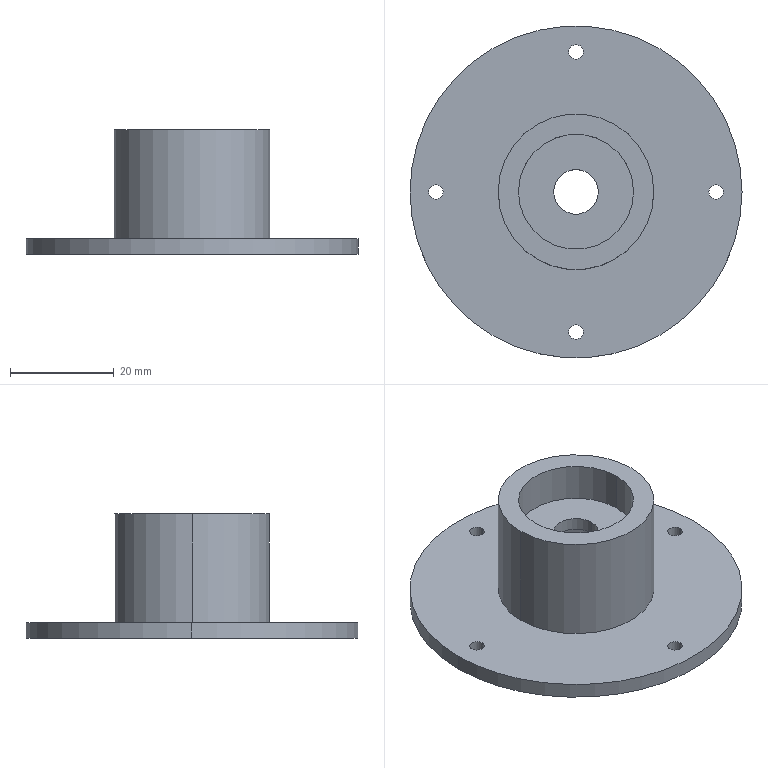Part | SolidWorks | features Fillet 1, HoleWzd 1, ICE 1, RevCut 1, Revolution 1 | 1 solid | 23 faces | box 64 x 64 x 24 mm | volume 13940 mm3 | cylinder 18 | plane 5 | commonest cylinder face diameters 2.8 x8 8.6 x2 22.2 x2 26 x2 30 x2 64 x2
STEP:
#1=CARTESIAN_POINT('',(-1.4,27.,0.));
#2=VERTEX_POINT('',#1);
#3=CARTESIAN_POINT('',(1.4,27.,0.));
#4=VERTEX_POINT('',#3);
#5=CARTESIAN_POINT('',(0.,27.,0.));
#6=DIRECTION('',(0.,0.,1.));
#7=DIRECTION('',(1.,0.,0.));
#8=AXIS2_PLACEMENT_3D('',#5,#6,#7);
#9=CIRCLE('',#8,1.4);
#10=EDGE_CURVE('',#2,#4,#9,.T.);
#11=ORIENTED_EDGE('',*,*,#10,.F.);
#12=CARTESIAN_POINT('',(-1.4,27.,3.));
#13=VERTEX_POINT('',#12);
#14=CARTESIAN_POINT('',(-1.4,27.,3.));
#15=DIRECTION('',(0.,0.,1.));
#16=VECTOR('',#15,1000.);
#17=LINE('',#14,#16);
#18=EDGE_CURVE('',#2,#13,#17,.T.);
#19=ORIENTED_EDGE('',*,*,#18,.T.);
#20=CARTESIAN_POINT('',(1.4,27.,3.));
#21=VERTEX_POINT('',#20);
#22=CARTESIAN_POINT('',(0.,27.,3.));
#23=DIRECTION('',(0.,0.,1.));
#24=DIRECTION('',(1.,0.,0.));
#25=AXIS2_PLACEMENT_3D('',#22,#23,#24);
#26=CIRCLE('',#25,1.4);
#27=EDGE_CURVE('',#13,#21,#26,.T.);
#28=ORIENTED_EDGE('',*,*,#27,.T.);
#29=CARTESIAN_POINT('',(1.4,27.,3.));
#30=DIRECTION('',(0.,0.,1.));
#31=VECTOR('',#30,1000.);
#32=LINE('',#29,#31);
#33=EDGE_CURVE('',#4,#21,#32,.T.);
#34=ORIENTED_EDGE('',*,*,#33,.F.);
#35=EDGE_LOOP('',(#11,#19,#28,#34));
#36=FACE_OUTER_BOUND('',#35,.T.);
#37=CARTESIAN_POINT('',(0.,27.,3.));
#38=DIRECTION('',(0.,0.,1.));
#39=DIRECTION('',(1.,0.,0.));
#40=AXIS2_PLACEMENT_3D('',#37,#38,#39);
#41=CYLINDRICAL_SURFACE('',#40,1.4);
#42=ADVANCED_FACE('',(#36),#41,.F.);
#43=CARTESIAN_POINT('',(-1.4,-27.,0.));
#44=VERTEX_POINT('',#43);
#45=CARTESIAN_POINT('',(1.4,-27.,0.));
#46=VERTEX_POINT('',#45);
#47=CARTESIAN_POINT('',(0.,-27.,0.));
#48=DIRECTION('',(0.,0.,1.));
#49=DIRECTION('',(1.,0.,0.));
#50=AXIS2_PLACEMENT_3D('',#47,#48,#49);
#51=CIRCLE('',#50,1.4);
#52=EDGE_CURVE('',#44,#46,#51,.T.);
#53=ORIENTED_EDGE('',*,*,#52,.F.);
#54=CARTESIAN_POINT('',(-1.4,-27.,3.));
#55=VERTEX_POINT('',#54);
#56=CARTESIAN_POINT('',(-1.4,-27.,3.));
#57=DIRECTION('',(0.,0.,1.));
#58=VECTOR('',#57,1000.);
#59=LINE('',#56,#58);
#60=EDGE_CURVE('',#44,#55,#59,.T.);
#61=ORIENTED_EDGE('',*,*,#60,.T.);
#62=CARTESIAN_POINT('',(1.4,-27.,3.));
#63=VERTEX_POINT('',#62);
#64=CARTESIAN_POINT('',(0.,-27.,3.));
#65=DIRECTION('',(0.,0.,1.));
#66=DIRECTION('',(1.,0.,0.));
#67=AXIS2_PLACEMENT_3D('',#64,#65,#66);
#68=CIRCLE('',#67,1.4);
#69=EDGE_CURVE('',#55,#63,#68,.T.);
#70=ORIENTED_EDGE('',*,*,#69,.T.);
#71=CARTESIAN_POINT('',(1.4,-27.,3.));
#72=DIRECTION('',(0.,0.,1.));
#73=VECTOR('',#72,1000.);
#74=LINE('',#71,#73);
#75=EDGE_CURVE('',#46,#63,#74,.T.);
#76=ORIENTED_EDGE('',*,*,#75,.F.);
#77=EDGE_LOOP('',(#53,#61,#70,#76));
#78=FACE_OUTER_BOUND('',#77,.T.);
#79=CARTESIAN_POINT('',(0.,-27.,3.));
#80=DIRECTION('',(0.,0.,1.));
#81=DIRECTION('',(1.,0.,0.));
#82=AXIS2_PLACEMENT_3D('',#79,#80,#81);
#83=CYLINDRICAL_SURFACE('',#82,1.4);
#84=ADVANCED_FACE('',(#78),#83,.F.);
#85=CARTESIAN_POINT('',(25.6,0.,0.));
#86=VERTEX_POINT('',#85);
#87=CARTESIAN_POINT('',(28.4,0.,0.));
#88=VERTEX_POINT('',#87);
#89=CARTESIAN_POINT('',(27.,0.,0.));
#90=DIRECTION('',(0.,0.,1.));
#91=DIRECTION('',(1.,0.,0.));
#92=AXIS2_PLACEMENT_3D('',#89,#90,#91);
#93=CIRCLE('',#92,1.4);
#94=EDGE_CURVE('',#86,#88,#93,.T.);
#95=ORIENTED_EDGE('',*,*,#94,.F.);
#96=CARTESIAN_POINT('',(25.6,0.,3.));
#97=VERTEX_POINT('',#96);
#98=CARTESIAN_POINT('',(25.6,0.,3.));
#99=DIRECTION('',(0.,0.,1.));
#100=VECTOR('',#99,1000.);
#101=LINE('',#98,#100);
#102=EDGE_CURVE('',#86,#97,#101,.T.);
#103=ORIENTED_EDGE('',*,*,#102,.T.);
#104=CARTESIAN_POINT('',(28.4,0.,3.));
#105=VERTEX_POINT('',#104);
#106=CARTESIAN_POINT('',(27.,0.,3.));
#107=DIRECTION('',(0.,0.,1.));
#108=DIRECTION('',(1.,0.,0.));
#109=AXIS2_PLACEMENT_3D('',#106,#107,#108);
#110=CIRCLE('',#109,1.4);
#111=EDGE_CURVE('',#97,#105,#110,.T.);
#112=ORIENTED_EDGE('',*,*,#111,.T.);
#113=CARTESIAN_POINT('',(28.4,0.,3.));
#114=DIRECTION('',(0.,0.,1.));
#115=VECTOR('',#114,1000.);
#116=LINE('',#113,#115);
#117=EDGE_CURVE('',#88,#105,#116,.T.);
#118=ORIENTED_EDGE('',*,*,#117,.F.);
#119=EDGE_LOOP('',(#95,#103,#112,#118));
#120=FACE_OUTER_BOUND('',#119,.T.);
#121=CARTESIAN_POINT('',(27.,0.,3.));
#122=DIRECTION('',(0.,0.,1.));
#123=DIRECTION('',(1.,0.,0.));
#124=AXIS2_PLACEMENT_3D('',#121,#122,#123);
#125=CYLINDRICAL_SURFACE('',#124,1.4);
#126=ADVANCED_FACE('',(#120),#125,.F.);
#127=CARTESIAN_POINT('',(-28.4,0.,0.));
#128=VERTEX_POINT('',#127);
#129=CARTESIAN_POINT('',(-25.6,0.,0.));
#130=VERTEX_POINT('',#129);
#131=CARTESIAN_POINT('',(-27.,0.,0.));
#132=DIRECTION('',(0.,0.,1.));
#133=DIRECTION('',(1.,0.,0.));
#134=AXIS2_PLACEMENT_3D('',#131,#132,#133);
#135=CIRCLE('',#134,1.4);
#136=EDGE_CURVE('',#128,#130,#135,.T.);
#137=ORIENTED_EDGE('',*,*,#136,.F.);
#138=CARTESIAN_POINT('',(-28.4,0.,3.));
#139=VERTEX_POINT('',#138);
#140=CARTESIAN_POINT('',(-28.4,0.,3.));
#141=DIRECTION('',(0.,0.,1.));
#142=VECTOR('',#141,1000.);
#143=LINE('',#140,#142);
#144=EDGE_CURVE('',#128,#139,#143,.T.);
#145=ORIENTED_EDGE('',*,*,#144,.T.);
#146=CARTESIAN_POINT('',(-25.6,0.,3.));
#147=VERTEX_POINT('',#146);
#148=CARTESIAN_POINT('',(-27.,0.,3.));
#149=DIRECTION('',(0.,0.,1.));
#150=DIRECTION('',(1.,0.,0.));
#151=AXIS2_PLACEMENT_3D('',#148,#149,#150);
#152=CIRCLE('',#151,1.4);
#153=EDGE_CURVE('',#139,#147,#152,.T.);
#154=ORIENTED_EDGE('',*,*,#153,.T.);
#155=CARTESIAN_POINT('',(-25.6,0.,3.));
#156=DIRECTION('',(0.,0.,1.));
#157=VECTOR('',#156,1000.);
#158=LINE('',#155,#157);
#159=EDGE_CURVE('',#130,#147,#158,.T.);
#160=ORIENTED_EDGE('',*,*,#159,.F.);
#161=EDGE_LOOP('',(#137,#145,#154,#160));
#162=FACE_OUTER_BOUND('',#161,.T.);
#163=CARTESIAN_POINT('',(-27.,0.,3.));
#164=DIRECTION('',(0.,0.,1.));
#165=DIRECTION('',(1.,0.,0.));
#166=AXIS2_PLACEMENT_3D('',#163,#164,#165);
#167=CYLINDRICAL_SURFACE('',#166,1.4);
#168=ADVANCED_FACE('',(#162),#167,.F.);
#169=CARTESIAN_POINT('',(-4.3,0.,14.));
#170=VERTEX_POINT('',#169);
#171=CARTESIAN_POINT('',(4.3,0.,14.));
#172=VERTEX_POINT('',#171);
#173=CARTESIAN_POINT('',(0.,0.,14.));
#174=DIRECTION('',(0.,0.,1.));
#175=DIRECTION('',(1.,0.,0.));
#176=AXIS2_PLACEMENT_3D('',#173,#174,#175);
#177=CIRCLE('',#176,4.3);
#178=EDGE_CURVE('',#170,#172,#177,.T.);
#179=ORIENTED_EDGE('',*,*,#178,.F.);
#180=CARTESIAN_POINT('',(-4.3,0.,16.5));
#181=VERTEX_POINT('',#180);
#182=CARTESIAN_POINT('',(-4.3,0.,0.));
#183=DIRECTION('',(0.,0.,1.));
#184=VECTOR('',#183,1000.);
#185=LINE('',#182,#184);
#186=EDGE_CURVE('',#170,#181,#185,.T.);
#187=ORIENTED_EDGE('',*,*,#186,.T.);
#188=CARTESIAN_POINT('',(4.3,0.,16.5));
#189=VERTEX_POINT('',#188);
#190=CARTESIAN_POINT('',(0.,0.,16.5));
#191=DIRECTION('',(0.,0.,1.));
#192=DIRECTION('',(1.,0.,0.));
#193=AXIS2_PLACEMENT_3D('',#190,#191,#192);
#194=CIRCLE('',#193,4.3);
#195=EDGE_CURVE('',#181,#189,#194,.T.);
#196=ORIENTED_EDGE('',*,*,#195,.T.);
#197=CARTESIAN_POINT('',(4.3,0.,0.));
#198=DIRECTION('',(0.,0.,1.));
#199=VECTOR('',#198,1000.);
#200=LINE('',#197,#199);
#201=EDGE_CURVE('',#172,#189,#200,.T.);
#202=ORIENTED_EDGE('',*,*,#201,.F.);
#203=EDGE_LOOP('',(#179,#187,#196,#202));
#204=FACE_OUTER_BOUND('',#203,.T.);
#205=CARTESIAN_POINT('',(0.,0.,0.));
#206=DIRECTION('',(0.,0.,1.));
#207=DIRECTION('',(1.,0.,0.));
#208=AXIS2_PLACEMENT_3D('',#205,#206,#207);
#209=CYLINDRICAL_SURFACE('',#208,4.3);
#210=ADVANCED_FACE('',(#204),#209,.F.);
#211=CARTESIAN_POINT('',(-11.1,0.,16.5));
#212=VERTEX_POINT('',#211);
#213=CARTESIAN_POINT('',(11.1,0.,16.5));
#214=VERTEX_POINT('',#213);
#215=CARTESIAN_POINT('',(0.,0.,16.5));
#216=DIRECTION('',(0.,0.,1.));
#217=DIRECTION('',(1.,0.,0.));
#218=AXIS2_PLACEMENT_3D('',#215,#216,#217);
#219=CIRCLE('',#218,11.1);
#220=EDGE_CURVE('',#212,#214,#219,.T.);
#221=ORIENTED_EDGE('',*,*,#220,.F.);
#222=CARTESIAN_POINT('',(-11.1,0.,24.));
#223=VERTEX_POINT('',#222);
#224=CARTESIAN_POINT('',(-11.1,0.,0.));
#225=DIRECTION('',(0.,0.,1.));
#226=VECTOR('',#225,1000.);
#227=LINE('',#224,#226);
#228=EDGE_CURVE('',#212,#223,#227,.T.);
#229=ORIENTED_EDGE('',*,*,#228,.T.);
#230=CARTESIAN_POINT('',(11.1,0.,24.));
#231=VERTEX_POINT('',#230);
#232=CARTESIAN_POINT('',(0.,0.,24.));
#233=DIRECTION('',(0.,0.,1.));
#234=DIRECTION('',(1.,0.,0.));
#235=AXIS2_PLACEMENT_3D('',#232,#233,#234);
#236=CIRCLE('',#235,11.1);
#237=EDGE_CURVE('',#223,#231,#236,.T.);
#238=ORIENTED_EDGE('',*,*,#237,.T.);
#239=CARTESIAN_POINT('',(11.1,0.,0.));
#240=DIRECTION('',(0.,0.,1.));
#241=VECTOR('',#240,1000.);
#242=LINE('',#239,#241);
#243=EDGE_CURVE('',#214,#231,#242,.T.);
#244=ORIENTED_EDGE('',*,*,#243,.F.);
#245=EDGE_LOOP('',(#221,#229,#238,#244));
#246=FACE_OUTER_BOUND('',#245,.T.);
#247=CARTESIAN_POINT('',(0.,0.,0.));
#248=DIRECTION('',(0.,0.,1.));
#249=DIRECTION('',(1.,0.,0.));
#250=AXIS2_PLACEMENT_3D('',#247,#248,#249);
#251=CYLINDRICAL_SURFACE('',#250,11.1);
#252=ADVANCED_FACE('',(#246),#251,.F.);
#253=CARTESIAN_POINT('',(-13.,0.,0.));
#254=VERTEX_POINT('',#253);
#255=CARTESIAN_POINT('',(13.,0.,0.));
#256=VERTEX_POINT('',#255);
#257=CARTESIAN_POINT('',(0.,0.,0.));
#258=DIRECTION('',(0.,0.,1.));
#259=DIRECTION('',(1.,0.,0.));
#260=AXIS2_PLACEMENT_3D('',#257,#258,#259);
#261=CIRCLE('',#260,13.);
#262=EDGE_CURVE('',#254,#256,#261,.T.);
#263=ORIENTED_EDGE('',*,*,#262,.F.);
#264=CARTESIAN_POINT('',(-13.,0.,14.));
#265=VERTEX_POINT('',#264);
#266=CARTESIAN_POINT('',(-13.,0.,0.));
#267=DIRECTION('',(0.,0.,1.));
#268=VECTOR('',#267,1000.);
#269=LINE('',#266,#268);
#270=EDGE_CURVE('',#254,#265,#269,.T.);
#271=ORIENTED_EDGE('',*,*,#270,.T.);
#272=CARTESIAN_POINT('',(13.,0.,14.));
#273=VERTEX_POINT('',#272);
#274=CARTESIAN_POINT('',(0.,0.,14.));
#275=DIRECTION('',(0.,0.,1.));
#276=DIRECTION('',(1.,0.,0.));
#277=AXIS2_PLACEMENT_3D('',#274,#275,#276);
#278=CIRCLE('',#277,13.);
#279=EDGE_CURVE('',#265,#273,#278,.T.);
#280=ORIENTED_EDGE('',*,*,#279,.T.);
#281=CARTESIAN_POINT('',(13.,0.,0.));
#282=DIRECTION('',(0.,0.,1.));
#283=VECTOR('',#282,1000.);
#284=LINE('',#281,#283);
#285=EDGE_CURVE('',#256,#273,#284,.T.);
#286=ORIENTED_EDGE('',*,*,#285,.F.);
#287=EDGE_LOOP('',(#263,#271,#280,#286));
#288=FACE_OUTER_BOUND('',#287,.T.);
#289=CARTESIAN_POINT('',(0.,0.,0.));
#290=DIRECTION('',(0.,0.,1.));
#291=DIRECTION('',(1.,0.,0.));
#292=AXIS2_PLACEMENT_3D('',#289,#290,#291);
#293=CYLINDRICAL_SURFACE('',#292,13.);
#294=ADVANCED_FACE('',(#288),#293,.F.);
#295=CARTESIAN_POINT('',(15.,0.,24.));
#296=VERTEX_POINT('',#295);
#297=CARTESIAN_POINT('',(-15.,0.,24.));
#298=VERTEX_POINT('',#297);
#299=CARTESIAN_POINT('',(0.,0.,24.));
#300=DIRECTION('',(0.,0.,1.));
#301=DIRECTION('',(1.,0.,0.));
#302=AXIS2_PLACEMENT_3D('',#299,#300,#301);
#303=CIRCLE('',#302,15.);
#304=EDGE_CURVE('',#296,#298,#303,.T.);
#305=ORIENTED_EDGE('',*,*,#304,.F.);
#306=CARTESIAN_POINT('',(15.,0.,3.));
#307=VERTEX_POINT('',#306);
#308=CARTESIAN_POINT('',(15.,0.,24.));
#309=DIRECTION('',(0.,0.,-1.));
#310=VECTOR('',#309,1000.);
#311=LINE('',#308,#310);
#312=EDGE_CURVE('',#296,#307,#311,.T.);
#313=ORIENTED_EDGE('',*,*,#312,.T.);
#314=CARTESIAN_POINT('',(-15.,0.,3.));
#315=VERTEX_POINT('',#314);
#316=CARTESIAN_POINT('',(0.,0.,3.));
#317=DIRECTION('',(0.,0.,1.));
#318=DIRECTION('',(1.,0.,0.));
#319=AXIS2_PLACEMENT_3D('',#316,#317,#318);
#320=CIRCLE('',#319,15.);
#321=EDGE_CURVE('',#307,#315,#320,.T.);
#322=ORIENTED_EDGE('',*,*,#321,.T.);
#323=CARTESIAN_POINT('',(-15.,0.,24.));
#324=DIRECTION('',(0.,0.,-1.));
#325=VECTOR('',#324,1000.);
#326=LINE('',#323,#325);
#327=EDGE_CURVE('',#298,#315,#326,.T.);
#328=ORIENTED_EDGE('',*,*,#327,.F.);
#329=EDGE_LOOP('',(#305,#313,#322,#328));
#330=FACE_OUTER_BOUND('',#329,.T.);
#331=CARTESIAN_POINT('',(0.,0.,24.));
#332=DIRECTION('',(0.,0.,-1.));
#333=DIRECTION('',(-1.,0.,0.));
#334=AXIS2_PLACEMENT_3D('',#331,#332,#333);
#335=CYLINDRICAL_SURFACE('',#334,15.);
#336=ADVANCED_FACE('',(#330),#335,.T.);
#337=CARTESIAN_POINT('',(32.,0.,0.));
#338=VERTEX_POINT('',#337);
#339=CARTESIAN_POINT('',(-32.,0.,0.));
#340=VERTEX_POINT('',#339);
#341=CARTESIAN_POINT('',(0.,0.,0.));
#342=DIRECTION('',(0.,0.,1.));
#343=DIRECTION('',(1.,0.,0.));
#344=AXIS2_PLACEMENT_3D('',#341,#342,#343);
#345=CIRCLE('',#344,32.);
#346=EDGE_CURVE('',#338,#340,#345,.T.);
#347=ORIENTED_EDGE('',*,*,#346,.T.);
#348=CARTESIAN_POINT('',(-32.,0.,3.));
#349=VERTEX_POINT('',#348);
#350=CARTESIAN_POINT('',(-32.,0.,0.));
#351=DIRECTION('',(0.,0.,1.));
#352=VECTOR('',#351,1000.);
#353=LINE('',#350,#352);
#354=EDGE_CURVE('',#340,#349,#353,.T.);
#355=ORIENTED_EDGE('',*,*,#354,.T.);
#356=CARTESIAN_POINT('',(32.,0.,3.));
#357=VERTEX_POINT('',#356);
#358=CARTESIAN_POINT('',(0.,0.,3.));
#359=DIRECTION('',(0.,0.,1.));
#360=DIRECTION('',(1.,0.,0.));
#361=AXIS2_PLACEMENT_3D('',#358,#359,#360);
#362=CIRCLE('',#361,32.);
#363=EDGE_CURVE('',#357,#349,#362,.T.);
#364=ORIENTED_EDGE('',*,*,#363,.F.);
#365=CARTESIAN_POINT('',(32.,0.,0.));
#366=DIRECTION('',(0.,0.,1.));
#367=VECTOR('',#366,1000.);
#368=LINE('',#365,#367);
#369=EDGE_CURVE('',#338,#357,#368,.T.);
#370=ORIENTED_EDGE('',*,*,#369,.F.);
#371=EDGE_LOOP('',(#347,#355,#364,#370));
#372=FACE_OUTER_BOUND('',#371,.T.);
#373=CARTESIAN_POINT('',(0.,0.,0.));
#374=DIRECTION('',(0.,0.,1.));
#375=DIRECTION('',(1.,0.,0.));
#376=AXIS2_PLACEMENT_3D('',#373,#374,#375);
#377=CYLINDRICAL_SURFACE('',#376,32.);
#378=ADVANCED_FACE('',(#372),#377,.T.);
#379=ORIENTED_EDGE('',*,*,#354,.F.);
#380=CARTESIAN_POINT('',(0.,0.,0.));
#381=DIRECTION('',(0.,0.,1.));
#382=DIRECTION('',(1.,0.,0.));
#383=AXIS2_PLACEMENT_3D('',#380,#381,#382);
#384=CIRCLE('',#383,32.);
#385=EDGE_CURVE('',#340,#338,#384,.T.);
#386=ORIENTED_EDGE('',*,*,#385,.T.);
#387=ORIENTED_EDGE('',*,*,#369,.T.);
#388=CARTESIAN_POINT('',(0.,0.,3.));
#389=DIRECTION('',(0.,0.,1.));
#390=DIRECTION('',(1.,0.,0.));
#391=AXIS2_PLACEMENT_3D('',#388,#389,#390);
#392=CIRCLE('',#391,32.);
#393=EDGE_CURVE('',#349,#357,#392,.T.);
#394=ORIENTED_EDGE('',*,*,#393,.F.);
#395=EDGE_LOOP('',(#379,#386,#387,#394));
#396=FACE_OUTER_BOUND('',#395,.T.);
#397=CARTESIAN_POINT('',(0.,0.,0.));
#398=DIRECTION('',(0.,0.,1.));
#399=DIRECTION('',(1.,0.,0.));
#400=AXIS2_PLACEMENT_3D('',#397,#398,#399);
#401=CYLINDRICAL_SURFACE('',#400,32.);
#402=ADVANCED_FACE('',(#396),#401,.T.);
#403=CARTESIAN_POINT('',(0.,27.,0.));
#404=DIRECTION('',(0.,0.,1.));
#405=DIRECTION('',(1.,0.,0.));
#406=AXIS2_PLACEMENT_3D('',#403,#404,#405);
#407=CIRCLE('',#406,1.4);
#408=EDGE_CURVE('',#4,#2,#407,.T.);
#409=ORIENTED_EDGE('',*,*,#408,.T.);
#410=ORIENTED_EDGE('',*,*,#10,.T.);
#411=EDGE_LOOP('',(#409,#410));
#412=FACE_BOUND('',#411,.T.);
#413=CARTESIAN_POINT('',(0.,-27.,0.));
#414=DIRECTION('',(0.,0.,1.));
#415=DIRECTION('',(1.,0.,0.));
#416=AXIS2_PLACEMENT_3D('',#413,#414,#415);
#417=CIRCLE('',#416,1.4);
#418=EDGE_CURVE('',#46,#44,#417,.T.);
#419=ORIENTED_EDGE('',*,*,#418,.T.);
#420=ORIENTED_EDGE('',*,*,#52,.T.);
#421=EDGE_LOOP('',(#419,#420));
#422=FACE_BOUND('',#421,.T.);
#423=CARTESIAN_POINT('',(27.,0.,0.));
#424=DIRECTION('',(0.,0.,1.));
#425=DIRECTION('',(1.,0.,0.));
#426=AXIS2_PLACEMENT_3D('',#423,#424,#425);
#427=CIRCLE('',#426,1.4);
#428=EDGE_CURVE('',#88,#86,#427,.T.);
#429=ORIENTED_EDGE('',*,*,#428,.T.);
#430=ORIENTED_EDGE('',*,*,#94,.T.);
#431=EDGE_LOOP('',(#429,#430));
#432=FACE_BOUND('',#431,.T.);
#433=CARTESIAN_POINT('',(-27.,0.,0.));
#434=DIRECTION('',(0.,0.,1.));
#435=DIRECTION('',(1.,0.,0.));
#436=AXIS2_PLACEMENT_3D('',#433,#434,#435);
#437=CIRCLE('',#436,1.4);
#438=EDGE_CURVE('',#130,#128,#437,.T.);
#439=ORIENTED_EDGE('',*,*,#438,.T.);
#440=ORIENTED_EDGE('',*,*,#136,.T.);
#441=EDGE_LOOP('',(#439,#440));
#442=FACE_BOUND('',#441,.T.);
#443=CARTESIAN_POINT('',(0.,0.,0.));
#444=DIRECTION('',(0.,0.,1.));
#445=DIRECTION('',(1.,0.,0.));
#446=AXIS2_PLACEMENT_3D('',#443,#444,#445);
#447=CIRCLE('',#446,13.);
#448=EDGE_CURVE('',#256,#254,#447,.T.);
#449=ORIENTED_EDGE('',*,*,#448,.T.);
#450=ORIENTED_EDGE('',*,*,#262,.T.);
#451=EDGE_LOOP('',(#449,#450));
#452=FACE_BOUND('',#451,.T.);
#453=ORIENTED_EDGE('',*,*,#346,.F.);
#454=ORIENTED_EDGE('',*,*,#385,.F.);
#455=EDGE_LOOP('',(#453,#454));
#456=FACE_OUTER_BOUND('',#455,.T.);
#457=CARTESIAN_POINT('',(32.,0.,0.));
#458=DIRECTION('',(0.,0.,-1.));
#459=DIRECTION('',(-1.,0.,0.));
#460=AXIS2_PLACEMENT_3D('',#457,#458,#459);
#461=PLANE('',#460);
#462=ADVANCED_FACE('',(#412,#422,#432,#442,#452,#456),#461,.T.);
#463=CARTESIAN_POINT('',(0.,27.,3.));
#464=DIRECTION('',(0.,0.,1.));
#465=DIRECTION('',(1.,0.,0.));
#466=AXIS2_PLACEMENT_3D('',#463,#464,#465);
#467=CIRCLE('',#466,1.4);
#468=EDGE_CURVE('',#21,#13,#467,.T.);
#469=ORIENTED_EDGE('',*,*,#468,.F.);
#470=ORIENTED_EDGE('',*,*,#27,.F.);
#471=EDGE_LOOP('',(#469,#470));
#472=FACE_BOUND('',#471,.T.);
#473=CARTESIAN_POINT('',(0.,-27.,3.));
#474=DIRECTION('',(0.,0.,1.));
#475=DIRECTION('',(1.,0.,0.));
#476=AXIS2_PLACEMENT_3D('',#473,#474,#475);
#477=CIRCLE('',#476,1.4);
#478=EDGE_CURVE('',#63,#55,#477,.T.);
#479=ORIENTED_EDGE('',*,*,#478,.F.);
#480=ORIENTED_EDGE('',*,*,#69,.F.);
#481=EDGE_LOOP('',(#479,#480));
#482=FACE_BOUND('',#481,.T.);
#483=CARTESIAN_POINT('',(27.,0.,3.));
#484=DIRECTION('',(0.,0.,1.));
#485=DIRECTION('',(1.,0.,0.));
#486=AXIS2_PLACEMENT_3D('',#483,#484,#485);
#487=CIRCLE('',#486,1.4);
#488=EDGE_CURVE('',#105,#97,#487,.T.);
#489=ORIENTED_EDGE('',*,*,#488,.F.);
#490=ORIENTED_EDGE('',*,*,#111,.F.);
#491=EDGE_LOOP('',(#489,#490));
#492=FACE_BOUND('',#491,.T.);
#493=CARTESIAN_POINT('',(-27.,0.,3.));
#494=DIRECTION('',(0.,0.,1.));
#495=DIRECTION('',(1.,0.,0.));
#496=AXIS2_PLACEMENT_3D('',#493,#494,#495);
#497=CIRCLE('',#496,1.4);
#498=EDGE_CURVE('',#147,#139,#497,.T.);
#499=ORIENTED_EDGE('',*,*,#498,.F.);
#500=ORIENTED_EDGE('',*,*,#153,.F.);
#501=EDGE_LOOP('',(#499,#500));
#502=FACE_BOUND('',#501,.T.);
#503=CARTESIAN_POINT('',(0.,0.,3.));
#504=DIRECTION('',(0.,0.,1.));
#505=DIRECTION('',(1.,0.,0.));
#506=AXIS2_PLACEMENT_3D('',#503,#504,#505);
#507=CIRCLE('',#506,15.);
#508=EDGE_CURVE('',#315,#307,#507,.T.);
#509=ORIENTED_EDGE('',*,*,#508,.F.);
#510=ORIENTED_EDGE('',*,*,#321,.F.);
#511=EDGE_LOOP('',(#509,#510));
#512=FACE_BOUND('',#511,.T.);
#513=ORIENTED_EDGE('',*,*,#363,.T.);
#514=ORIENTED_EDGE('',*,*,#393,.T.);
#515=EDGE_LOOP('',(#513,#514));
#516=FACE_OUTER_BOUND('',#515,.T.);
#517=CARTESIAN_POINT('',(0.,0.,3.));
#518=DIRECTION('',(0.,0.,1.));
#519=DIRECTION('',(1.,0.,0.));
#520=AXIS2_PLACEMENT_3D('',#517,#518,#519);
#521=PLANE('',#520);
#522=ADVANCED_FACE('',(#472,#482,#492,#502,#512,#516),#521,.T.);
#523=ORIENTED_EDGE('',*,*,#312,.F.);
#524=CARTESIAN_POINT('',(0.,0.,24.));
#525=DIRECTION('',(0.,0.,1.));
#526=DIRECTION('',(1.,0.,0.));
#527=AXIS2_PLACEMENT_3D('',#524,#525,#526);
#528=CIRCLE('',#527,15.);
#529=EDGE_CURVE('',#298,#296,#528,.T.);
#530=ORIENTED_EDGE('',*,*,#529,.F.);
#531=ORIENTED_EDGE('',*,*,#327,.T.);
#532=ORIENTED_EDGE('',*,*,#508,.T.);
#533=EDGE_LOOP('',(#523,#530,#531,#532));
#534=FACE_OUTER_BOUND('',#533,.T.);
#535=CARTESIAN_POINT('',(0.,0.,24.));
#536=DIRECTION('',(0.,0.,-1.));
#537=DIRECTION('',(-1.,0.,0.));
#538=AXIS2_PLACEMENT_3D('',#535,#536,#537);
#539=CYLINDRICAL_SURFACE('',#538,15.);
#540=ADVANCED_FACE('',(#534),#539,.T.);
#541=CARTESIAN_POINT('',(0.,0.,24.));
#542=DIRECTION('',(0.,0.,1.));
#543=DIRECTION('',(1.,0.,0.));
#544=AXIS2_PLACEMENT_3D('',#541,#542,#543);
#545=CIRCLE('',#544,11.1);
#546=EDGE_CURVE('',#231,#223,#545,.T.);
#547=ORIENTED_EDGE('',*,*,#546,.F.);
#548=ORIENTED_EDGE('',*,*,#237,.F.);
#549=EDGE_LOOP('',(#547,#548));
#550=FACE_BOUND('',#549,.T.);
#551=ORIENTED_EDGE('',*,*,#529,.T.);
#552=ORIENTED_EDGE('',*,*,#304,.T.);
#553=EDGE_LOOP('',(#551,#552));
#554=FACE_OUTER_BOUND('',#553,.T.);
#555=CARTESIAN_POINT('',(0.,0.,24.));
#556=DIRECTION('',(0.,0.,1.));
#557=DIRECTION('',(1.,0.,0.));
#558=AXIS2_PLACEMENT_3D('',#555,#556,#557);
#559=PLANE('',#558);
#560=ADVANCED_FACE('',(#550,#554),#559,.T.);
#561=ORIENTED_EDGE('',*,*,#270,.F.);
#562=ORIENTED_EDGE('',*,*,#448,.F.);
#563=ORIENTED_EDGE('',*,*,#285,.T.);
#564=CARTESIAN_POINT('',(0.,0.,14.));
#565=DIRECTION('',(0.,0.,1.));
#566=DIRECTION('',(1.,0.,0.));
#567=AXIS2_PLACEMENT_3D('',#564,#565,#566);
#568=CIRCLE('',#567,13.);
#569=EDGE_CURVE('',#273,#265,#568,.T.);
#570=ORIENTED_EDGE('',*,*,#569,.T.);
#571=EDGE_LOOP('',(#561,#562,#563,#570));
#572=FACE_OUTER_BOUND('',#571,.T.);
#573=CARTESIAN_POINT('',(0.,0.,0.));
#574=DIRECTION('',(0.,0.,1.));
#575=DIRECTION('',(1.,0.,0.));
#576=AXIS2_PLACEMENT_3D('',#573,#574,#575);
#577=CYLINDRICAL_SURFACE('',#576,13.);
#578=ADVANCED_FACE('',(#572),#577,.F.);
#579=ORIENTED_EDGE('',*,*,#228,.F.);
#580=CARTESIAN_POINT('',(0.,0.,16.5));
#581=DIRECTION('',(0.,0.,1.));
#582=DIRECTION('',(1.,0.,0.));
#583=AXIS2_PLACEMENT_3D('',#580,#581,#582);
#584=CIRCLE('',#583,11.1);
#585=EDGE_CURVE('',#214,#212,#584,.T.);
#586=ORIENTED_EDGE('',*,*,#585,.F.);
#587=ORIENTED_EDGE('',*,*,#243,.T.);
#588=ORIENTED_EDGE('',*,*,#546,.T.);
#589=EDGE_LOOP('',(#579,#586,#587,#588));
#590=FACE_OUTER_BOUND('',#589,.T.);
#591=CARTESIAN_POINT('',(0.,0.,0.));
#592=DIRECTION('',(0.,0.,1.));
#593=DIRECTION('',(1.,0.,0.));
#594=AXIS2_PLACEMENT_3D('',#591,#592,#593);
#595=CYLINDRICAL_SURFACE('',#594,11.1);
#596=ADVANCED_FACE('',(#590),#595,.F.);
#597=CARTESIAN_POINT('',(0.,0.,16.5));
#598=DIRECTION('',(0.,0.,1.));
#599=DIRECTION('',(1.,0.,0.));
#600=AXIS2_PLACEMENT_3D('',#597,#598,#599);
#601=CIRCLE('',#600,4.3);
#602=EDGE_CURVE('',#189,#181,#601,.T.);
#603=ORIENTED_EDGE('',*,*,#602,.F.);
#604=ORIENTED_EDGE('',*,*,#195,.F.);
#605=EDGE_LOOP('',(#603,#604));
#606=FACE_BOUND('',#605,.T.);
#607=ORIENTED_EDGE('',*,*,#585,.T.);
#608=ORIENTED_EDGE('',*,*,#220,.T.);
#609=EDGE_LOOP('',(#607,#608));
#610=FACE_OUTER_BOUND('',#609,.T.);
#611=CARTESIAN_POINT('',(11.1,0.,16.5));
#612=DIRECTION('',(0.,0.,-1.));
#613=DIRECTION('',(-1.,0.,0.));
#614=AXIS2_PLACEMENT_3D('',#611,#612,#613);
#615=PLANE('',#614);
#616=ADVANCED_FACE('',(#606,#610),#615,.F.);
#617=ORIENTED_EDGE('',*,*,#186,.F.);
#618=CARTESIAN_POINT('',(0.,0.,14.));
#619=DIRECTION('',(0.,0.,1.));
#620=DIRECTION('',(1.,0.,0.));
#621=AXIS2_PLACEMENT_3D('',#618,#619,#620);
#622=CIRCLE('',#621,4.3);
#623=EDGE_CURVE('',#172,#170,#622,.T.);
#624=ORIENTED_EDGE('',*,*,#623,.F.);
#625=ORIENTED_EDGE('',*,*,#201,.T.);
#626=ORIENTED_EDGE('',*,*,#602,.T.);
#627=EDGE_LOOP('',(#617,#624,#625,#626));
#628=FACE_OUTER_BOUND('',#627,.T.);
#629=CARTESIAN_POINT('',(0.,0.,0.));
#630=DIRECTION('',(0.,0.,1.));
#631=DIRECTION('',(1.,0.,0.));
#632=AXIS2_PLACEMENT_3D('',#629,#630,#631);
#633=CYLINDRICAL_SURFACE('',#632,4.3);
#634=ADVANCED_FACE('',(#628),#633,.F.);
#635=ORIENTED_EDGE('',*,*,#569,.F.);
#636=ORIENTED_EDGE('',*,*,#279,.F.);
#637=EDGE_LOOP('',(#635,#636));
#638=FACE_OUTER_BOUND('',#637,.T.);
#639=ORIENTED_EDGE('',*,*,#623,.T.);
#640=ORIENTED_EDGE('',*,*,#178,.T.);
#641=EDGE_LOOP('',(#639,#640));
#642=FACE_BOUND('',#641,.T.);
#643=CARTESIAN_POINT('',(4.3,0.,14.));
#644=DIRECTION('',(0.,0.,1.));
#645=DIRECTION('',(1.,0.,0.));
#646=AXIS2_PLACEMENT_3D('',#643,#644,#645);
#647=PLANE('',#646);
#648=ADVANCED_FACE('',(#638,#642),#647,.F.);
#649=ORIENTED_EDGE('',*,*,#144,.F.);
#650=ORIENTED_EDGE('',*,*,#438,.F.);
#651=ORIENTED_EDGE('',*,*,#159,.T.);
#652=ORIENTED_EDGE('',*,*,#498,.T.);
#653=EDGE_LOOP('',(#649,#650,#651,#652));
#654=FACE_OUTER_BOUND('',#653,.T.);
#655=CARTESIAN_POINT('',(-27.,0.,3.));
#656=DIRECTION('',(0.,0.,1.));
#657=DIRECTION('',(1.,0.,0.));
#658=AXIS2_PLACEMENT_3D('',#655,#656,#657);
#659=CYLINDRICAL_SURFACE('',#658,1.4);
#660=ADVANCED_FACE('',(#654),#659,.F.);
#661=ORIENTED_EDGE('',*,*,#102,.F.);
#662=ORIENTED_EDGE('',*,*,#428,.F.);
#663=ORIENTED_EDGE('',*,*,#117,.T.);
#664=ORIENTED_EDGE('',*,*,#488,.T.);
#665=EDGE_LOOP('',(#661,#662,#663,#664));
#666=FACE_OUTER_BOUND('',#665,.T.);
#667=CARTESIAN_POINT('',(27.,0.,3.));
#668=DIRECTION('',(0.,0.,1.));
#669=DIRECTION('',(1.,0.,0.));
#670=AXIS2_PLACEMENT_3D('',#667,#668,#669);
#671=CYLINDRICAL_SURFACE('',#670,1.4);
#672=ADVANCED_FACE('',(#666),#671,.F.);
#673=ORIENTED_EDGE('',*,*,#60,.F.);
#674=ORIENTED_EDGE('',*,*,#418,.F.);
#675=ORIENTED_EDGE('',*,*,#75,.T.);
#676=ORIENTED_EDGE('',*,*,#478,.T.);
#677=EDGE_LOOP('',(#673,#674,#675,#676));
#678=FACE_OUTER_BOUND('',#677,.T.);
#679=CARTESIAN_POINT('',(0.,-27.,3.));
#680=DIRECTION('',(0.,0.,1.));
#681=DIRECTION('',(1.,0.,0.));
#682=AXIS2_PLACEMENT_3D('',#679,#680,#681);
#683=CYLINDRICAL_SURFACE('',#682,1.4);
#684=ADVANCED_FACE('',(#678),#683,.F.);
#685=ORIENTED_EDGE('',*,*,#18,.F.);
#686=ORIENTED_EDGE('',*,*,#408,.F.);
#687=ORIENTED_EDGE('',*,*,#33,.T.);
#688=ORIENTED_EDGE('',*,*,#468,.T.);
#689=EDGE_LOOP('',(#685,#686,#687,#688));
#690=FACE_OUTER_BOUND('',#689,.T.);
#691=CARTESIAN_POINT('',(0.,27.,3.));
#692=DIRECTION('',(0.,0.,1.));
#693=DIRECTION('',(1.,0.,0.));
#694=AXIS2_PLACEMENT_3D('',#691,#692,#693);
#695=CYLINDRICAL_SURFACE('',#694,1.4);
#696=ADVANCED_FACE('',(#690),#695,.F.);
#697=CLOSED_SHELL('',(#42,#84,#126,#168,#210,#252,#294,#336,#378,#402,#462,#522,#540,#560,#578,#596,#616,#634,#648,#660,#672,#684,#696));
#698=MANIFOLD_SOLID_BREP('',#697);
#699=CARTESIAN_POINT('',(0.,0.,0.));
#700=DIRECTION('',(0.,0.,1.));
#701=DIRECTION('',(1.,0.,0.));
#702=AXIS2_PLACEMENT_3D('',#699,#700,#701);
#703=(LENGTH_UNIT()NAMED_UNIT(*)SI_UNIT(.MILLI.,.METRE.));
#704=UNCERTAINTY_MEASURE_WITH_UNIT(LENGTH_MEASURE(0.00001),#703,'','');
#705=(NAMED_UNIT(*)PLANE_ANGLE_UNIT()SI_UNIT($,.RADIAN.));
#706=(NAMED_UNIT(*)SI_UNIT($,.STERADIAN.)SOLID_ANGLE_UNIT());
#707=(GEOMETRIC_REPRESENTATION_CONTEXT(3)GLOBAL_UNCERTAINTY_ASSIGNED_CONTEXT((#704))GLOBAL_UNIT_ASSIGNED_CONTEXT((#703,#705,#706))REPRESENTATION_CONTEXT('',''));
#708=ADVANCED_BREP_SHAPE_REPRESENTATION('',(#698,#702),#707);